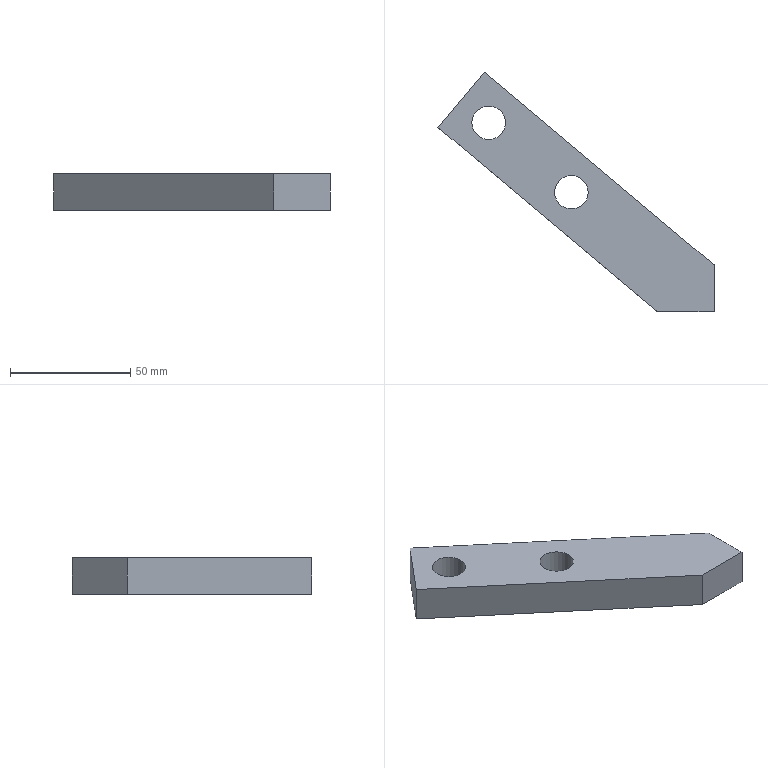Part | NX | features solid 2 | 1 solid | 9 faces | box 115.039 x 99.86 x 15 mm | volume 53844 mm3 | plane 7 | cylinder 2 | commonest cylinder face diameters 14 x2
STEP:
#1=CARTESIAN_POINT('',(-90.057,89.802,0.));
#2=VERTEX_POINT('',#1);
#3=CARTESIAN_POINT('',(-97.057,89.802,0.));
#4=DIRECTION('',(0.,0.,1.));
#5=DIRECTION('',(1.,0.,0.));
#6=AXIS2_PLACEMENT_3D('',#3,#4,#5);
#7=CIRCLE('',#6,7.);
#8=EDGE_CURVE('',#2,#2,#7,.T.);
#9=ORIENTED_EDGE('',*,*,#8,.F.);
#10=EDGE_LOOP('',(#9));
#11=FACE_BOUND('',#10,.T.);
#12=CARTESIAN_POINT('',(-37.623,59.512,0.));
#13=VERTEX_POINT('',#12);
#14=CARTESIAN_POINT('',(-37.623,40.,0.));
#15=VERTEX_POINT('',#14);
#16=CARTESIAN_POINT('',(-37.623,91.651,0.));
#17=DIRECTION('',(0.,-1.,0.));
#18=VECTOR('',#17,1000.);
#19=LINE('',#16,#18);
#20=EDGE_CURVE('',#13,#15,#19,.T.);
#21=ORIENTED_EDGE('',*,*,#20,.F.);
#22=CARTESIAN_POINT('',(-133.378,139.86,0.));
#23=VERTEX_POINT('',#22);
#24=CARTESIAN_POINT('',(-75.925,91.651,0.));
#25=DIRECTION('',(-0.766,0.6428,0.));
#26=VECTOR('',#25,1000.);
#27=LINE('',#24,#26);
#28=EDGE_CURVE('',#13,#23,#27,.T.);
#29=ORIENTED_EDGE('',*,*,#28,.T.);
#30=CARTESIAN_POINT('',(-152.662,116.879,0.));
#31=VERTEX_POINT('',#30);
#32=CARTESIAN_POINT('',(-133.378,139.86,0.));
#33=DIRECTION('',(-0.6428,-0.766,0.));
#34=VECTOR('',#33,1000.);
#35=LINE('',#32,#34);
#36=EDGE_CURVE('',#23,#31,#35,.T.);
#37=ORIENTED_EDGE('',*,*,#36,.T.);
#38=CARTESIAN_POINT('',(-61.041,40.,0.));
#39=VERTEX_POINT('',#38);
#40=CARTESIAN_POINT('',(-95.209,68.67,0.));
#41=DIRECTION('',(-0.766,0.6428,0.));
#42=VECTOR('',#41,1000.);
#43=LINE('',#40,#42);
#44=EDGE_CURVE('',#39,#31,#43,.T.);
#45=ORIENTED_EDGE('',*,*,#44,.F.);
#46=CARTESIAN_POINT('',(-37.623,40.,0.));
#47=DIRECTION('',(1.,0.,0.));
#48=VECTOR('',#47,1000.);
#49=LINE('',#46,#48);
#50=EDGE_CURVE('',#15,#39,#49,.F.);
#51=ORIENTED_EDGE('',*,*,#50,.F.);
#52=EDGE_LOOP('',(#21,#29,#37,#45,#51));
#53=FACE_BOUND('',#52,.T.);
#54=CARTESIAN_POINT('',(-124.529,118.728,0.));
#55=VERTEX_POINT('',#54);
#56=CARTESIAN_POINT('',(-131.529,118.728,0.));
#57=DIRECTION('',(0.,0.,1.));
#58=DIRECTION('',(1.,0.,0.));
#59=AXIS2_PLACEMENT_3D('',#56,#57,#58);
#60=CIRCLE('',#59,7.);
#61=EDGE_CURVE('',#55,#55,#60,.F.);
#62=ORIENTED_EDGE('',*,*,#61,.T.);
#63=EDGE_LOOP('',(#62));
#64=FACE_BOUND('',#63,.T.);
#65=CARTESIAN_POINT('',(-75.925,91.651,0.));
#66=DIRECTION('',(0.,0.,1.));
#67=DIRECTION('',(1.,0.,0.));
#68=AXIS2_PLACEMENT_3D('',#65,#66,#67);
#69=PLANE('',#68);
#70=ADVANCED_FACE('',(#11,#53,#64),#69,.T.);
#71=CARTESIAN_POINT('',(-90.057,89.802,-15.));
#72=VERTEX_POINT('',#71);
#73=CARTESIAN_POINT('',(-97.057,89.802,-15.));
#74=DIRECTION('',(0.,0.,1.));
#75=DIRECTION('',(1.,0.,0.));
#76=AXIS2_PLACEMENT_3D('',#73,#74,#75);
#77=CIRCLE('',#76,7.);
#78=EDGE_CURVE('',#72,#72,#77,.T.);
#79=ORIENTED_EDGE('',*,*,#78,.T.);
#80=EDGE_LOOP('',(#79));
#81=FACE_BOUND('',#80,.T.);
#82=CARTESIAN_POINT('',(-37.623,59.512,-15.));
#83=VERTEX_POINT('',#82);
#84=CARTESIAN_POINT('',(-133.378,139.86,-15.));
#85=VERTEX_POINT('',#84);
#86=CARTESIAN_POINT('',(-75.925,91.651,-15.));
#87=DIRECTION('',(-0.766,0.6428,0.));
#88=VECTOR('',#87,1000.);
#89=LINE('',#86,#88);
#90=EDGE_CURVE('',#83,#85,#89,.T.);
#91=ORIENTED_EDGE('',*,*,#90,.F.);
#92=CARTESIAN_POINT('',(-37.623,40.,-15.));
#93=VERTEX_POINT('',#92);
#94=CARTESIAN_POINT('',(-37.623,91.651,-15.));
#95=DIRECTION('',(0.,-1.,0.));
#96=VECTOR('',#95,1000.);
#97=LINE('',#94,#96);
#98=EDGE_CURVE('',#83,#93,#97,.T.);
#99=ORIENTED_EDGE('',*,*,#98,.T.);
#100=CARTESIAN_POINT('',(-61.041,40.,-15.));
#101=VERTEX_POINT('',#100);
#102=CARTESIAN_POINT('',(-37.623,40.,-15.));
#103=DIRECTION('',(1.,0.,0.));
#104=VECTOR('',#103,1000.);
#105=LINE('',#102,#104);
#106=EDGE_CURVE('',#93,#101,#105,.F.);
#107=ORIENTED_EDGE('',*,*,#106,.T.);
#108=CARTESIAN_POINT('',(-152.662,116.879,-15.));
#109=VERTEX_POINT('',#108);
#110=CARTESIAN_POINT('',(-95.209,68.67,-15.));
#111=DIRECTION('',(-0.766,0.6428,0.));
#112=VECTOR('',#111,1000.);
#113=LINE('',#110,#112);
#114=EDGE_CURVE('',#101,#109,#113,.T.);
#115=ORIENTED_EDGE('',*,*,#114,.T.);
#116=CARTESIAN_POINT('',(-133.378,139.86,-15.));
#117=DIRECTION('',(-0.6428,-0.766,0.));
#118=VECTOR('',#117,1000.);
#119=LINE('',#116,#118);
#120=EDGE_CURVE('',#85,#109,#119,.T.);
#121=ORIENTED_EDGE('',*,*,#120,.F.);
#122=EDGE_LOOP('',(#91,#99,#107,#115,#121));
#123=FACE_BOUND('',#122,.T.);
#124=CARTESIAN_POINT('',(-124.529,118.728,-15.));
#125=VERTEX_POINT('',#124);
#126=CARTESIAN_POINT('',(-131.529,118.728,-15.));
#127=DIRECTION('',(0.,0.,1.));
#128=DIRECTION('',(1.,0.,0.));
#129=AXIS2_PLACEMENT_3D('',#126,#127,#128);
#130=CIRCLE('',#129,7.);
#131=EDGE_CURVE('',#125,#125,#130,.F.);
#132=ORIENTED_EDGE('',*,*,#131,.F.);
#133=EDGE_LOOP('',(#132));
#134=FACE_BOUND('',#133,.T.);
#135=CARTESIAN_POINT('',(-75.925,91.651,-15.));
#136=DIRECTION('',(0.,0.,1.));
#137=DIRECTION('',(1.,0.,0.));
#138=AXIS2_PLACEMENT_3D('',#135,#136,#137);
#139=PLANE('',#138);
#140=ADVANCED_FACE('',(#81,#123,#134),#139,.F.);
#141=CARTESIAN_POINT('',(-37.623,59.512,-15.));
#142=DIRECTION('',(0.,0.,1.));
#143=VECTOR('',#142,1000.);
#144=LINE('',#141,#143);
#145=EDGE_CURVE('',#83,#13,#144,.T.);
#146=ORIENTED_EDGE('',*,*,#145,.F.);
#147=ORIENTED_EDGE('',*,*,#90,.T.);
#148=CARTESIAN_POINT('',(-133.378,139.86,-15.));
#149=DIRECTION('',(0.,0.,1.));
#150=VECTOR('',#149,1000.);
#151=LINE('',#148,#150);
#152=EDGE_CURVE('',#85,#23,#151,.T.);
#153=ORIENTED_EDGE('',*,*,#152,.T.);
#154=ORIENTED_EDGE('',*,*,#28,.F.);
#155=EDGE_LOOP('',(#146,#147,#153,#154));
#156=FACE_BOUND('',#155,.T.);
#157=CARTESIAN_POINT('',(-75.925,91.651,-15.));
#158=DIRECTION('',(0.6428,0.766,0.));
#159=DIRECTION('',(-0.766,0.6428,0.));
#160=AXIS2_PLACEMENT_3D('',#157,#158,#159);
#161=PLANE('',#160);
#162=ADVANCED_FACE('',(#156),#161,.T.);
#163=ORIENTED_EDGE('',*,*,#152,.F.);
#164=ORIENTED_EDGE('',*,*,#120,.T.);
#165=CARTESIAN_POINT('',(-152.662,116.879,-15.));
#166=DIRECTION('',(0.,0.,1.));
#167=VECTOR('',#166,1000.);
#168=LINE('',#165,#167);
#169=EDGE_CURVE('',#109,#31,#168,.T.);
#170=ORIENTED_EDGE('',*,*,#169,.T.);
#171=ORIENTED_EDGE('',*,*,#36,.F.);
#172=EDGE_LOOP('',(#163,#164,#170,#171));
#173=FACE_BOUND('',#172,.T.);
#174=CARTESIAN_POINT('',(-133.378,139.86,-15.));
#175=DIRECTION('',(-0.766,0.6428,0.));
#176=DIRECTION('',(-0.6428,-0.766,0.));
#177=AXIS2_PLACEMENT_3D('',#174,#175,#176);
#178=PLANE('',#177);
#179=ADVANCED_FACE('',(#173),#178,.T.);
#180=ORIENTED_EDGE('',*,*,#169,.F.);
#181=ORIENTED_EDGE('',*,*,#114,.F.);
#182=CARTESIAN_POINT('',(-61.041,40.,-15.));
#183=DIRECTION('',(0.,0.,1.));
#184=VECTOR('',#183,1000.);
#185=LINE('',#182,#184);
#186=EDGE_CURVE('',#101,#39,#185,.T.);
#187=ORIENTED_EDGE('',*,*,#186,.T.);
#188=ORIENTED_EDGE('',*,*,#44,.T.);
#189=EDGE_LOOP('',(#180,#181,#187,#188));
#190=FACE_BOUND('',#189,.T.);
#191=CARTESIAN_POINT('',(-95.209,68.67,-15.));
#192=DIRECTION('',(0.6428,0.766,0.));
#193=DIRECTION('',(-0.766,0.6428,0.));
#194=AXIS2_PLACEMENT_3D('',#191,#192,#193);
#195=PLANE('',#194);
#196=ADVANCED_FACE('',(#190),#195,.F.);
#197=CARTESIAN_POINT('',(-37.623,40.,-15.));
#198=DIRECTION('',(0.,0.,-1.));
#199=VECTOR('',#198,1000.);
#200=LINE('',#197,#199);
#201=EDGE_CURVE('',#93,#15,#200,.F.);
#202=ORIENTED_EDGE('',*,*,#201,.T.);
#203=ORIENTED_EDGE('',*,*,#50,.T.);
#204=ORIENTED_EDGE('',*,*,#186,.F.);
#205=ORIENTED_EDGE('',*,*,#106,.F.);
#206=EDGE_LOOP('',(#202,#203,#204,#205));
#207=FACE_BOUND('',#206,.T.);
#208=CARTESIAN_POINT('',(-37.623,40.,-15.));
#209=DIRECTION('',(0.,1.,0.));
#210=DIRECTION('',(0.,0.,1.));
#211=AXIS2_PLACEMENT_3D('',#208,#209,#210);
#212=PLANE('',#211);
#213=ADVANCED_FACE('',(#207),#212,.F.);
#214=ORIENTED_EDGE('',*,*,#145,.T.);
#215=ORIENTED_EDGE('',*,*,#20,.T.);
#216=ORIENTED_EDGE('',*,*,#201,.F.);
#217=ORIENTED_EDGE('',*,*,#98,.F.);
#218=EDGE_LOOP('',(#214,#215,#216,#217));
#219=FACE_BOUND('',#218,.T.);
#220=CARTESIAN_POINT('',(-37.623,70.,-15.));
#221=DIRECTION('',(-1.,0.,0.));
#222=DIRECTION('',(0.,0.,1.));
#223=AXIS2_PLACEMENT_3D('',#220,#221,#222);
#224=PLANE('',#223);
#225=ADVANCED_FACE('',(#219),#224,.F.);
#226=ORIENTED_EDGE('',*,*,#61,.F.);
#227=EDGE_LOOP('',(#226));
#228=FACE_BOUND('',#227,.T.);
#229=ORIENTED_EDGE('',*,*,#131,.T.);
#230=EDGE_LOOP('',(#229));
#231=FACE_BOUND('',#230,.T.);
#232=CARTESIAN_POINT('',(-131.529,118.728,-215.));
#233=DIRECTION('',(0.,0.,1.));
#234=DIRECTION('',(1.,0.,0.));
#235=AXIS2_PLACEMENT_3D('',#232,#233,#234);
#236=CYLINDRICAL_SURFACE('',#235,7.);
#237=ADVANCED_FACE('',(#228,#231),#236,.F.);
#238=ORIENTED_EDGE('',*,*,#8,.T.);
#239=EDGE_LOOP('',(#238));
#240=FACE_BOUND('',#239,.T.);
#241=ORIENTED_EDGE('',*,*,#78,.F.);
#242=EDGE_LOOP('',(#241));
#243=FACE_BOUND('',#242,.T.);
#244=CARTESIAN_POINT('',(-97.057,89.802,-215.));
#245=DIRECTION('',(0.,0.,1.));
#246=DIRECTION('',(1.,0.,0.));
#247=AXIS2_PLACEMENT_3D('',#244,#245,#246);
#248=CYLINDRICAL_SURFACE('',#247,7.);
#249=ADVANCED_FACE('',(#240,#243),#248,.F.);
#250=CLOSED_SHELL('',(#70,#140,#162,#179,#196,#213,#225,#237,#249));
#251=MANIFOLD_SOLID_BREP('',#250);
#252=(LENGTH_UNIT()NAMED_UNIT(*)SI_UNIT(.MILLI.,.METRE.));
#253=UNCERTAINTY_MEASURE_WITH_UNIT(LENGTH_MEASURE(0.00001),#252,'','');
#254=(NAMED_UNIT(*)PLANE_ANGLE_UNIT()SI_UNIT($,.RADIAN.));
#255=(NAMED_UNIT(*)SI_UNIT($,.STERADIAN.)SOLID_ANGLE_UNIT());
#256=(GEOMETRIC_REPRESENTATION_CONTEXT(3)GLOBAL_UNCERTAINTY_ASSIGNED_CONTEXT((#253))GLOBAL_UNIT_ASSIGNED_CONTEXT((#252,#254,#255))REPRESENTATION_CONTEXT('',''));
#257=ADVANCED_BREP_SHAPE_REPRESENTATION('',(#251),#256);